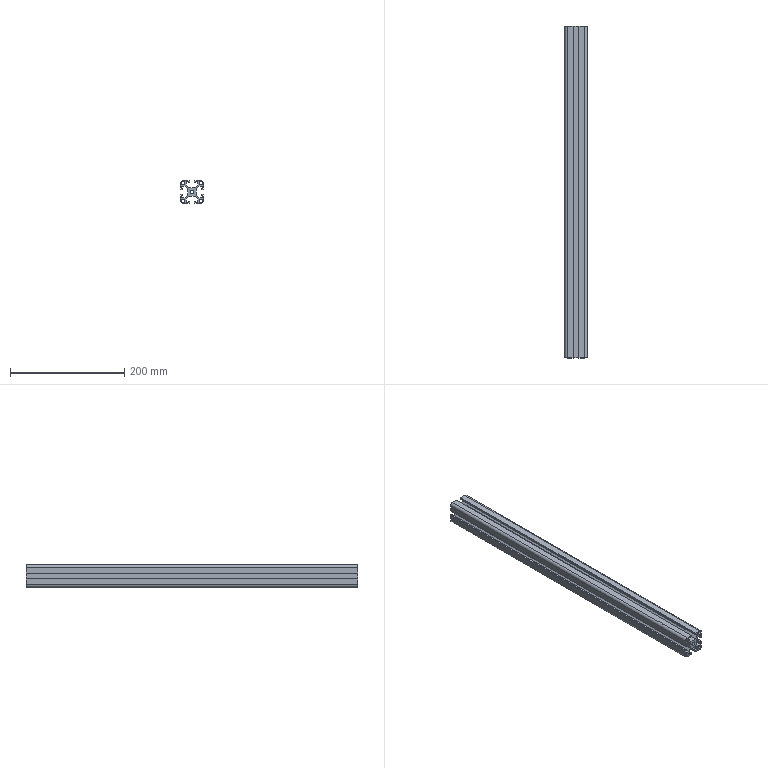Part | SolidWorks | features WeldMemberFeat 1, WeldmentFeature 1 | 1 solid | 92 faces | box 40 x 580 x 40 mm | volume 350809 mm3 | plane 78 | cylinder 14 | commonest cylinder face diameters 6 x8 9 x4 6.8 x2